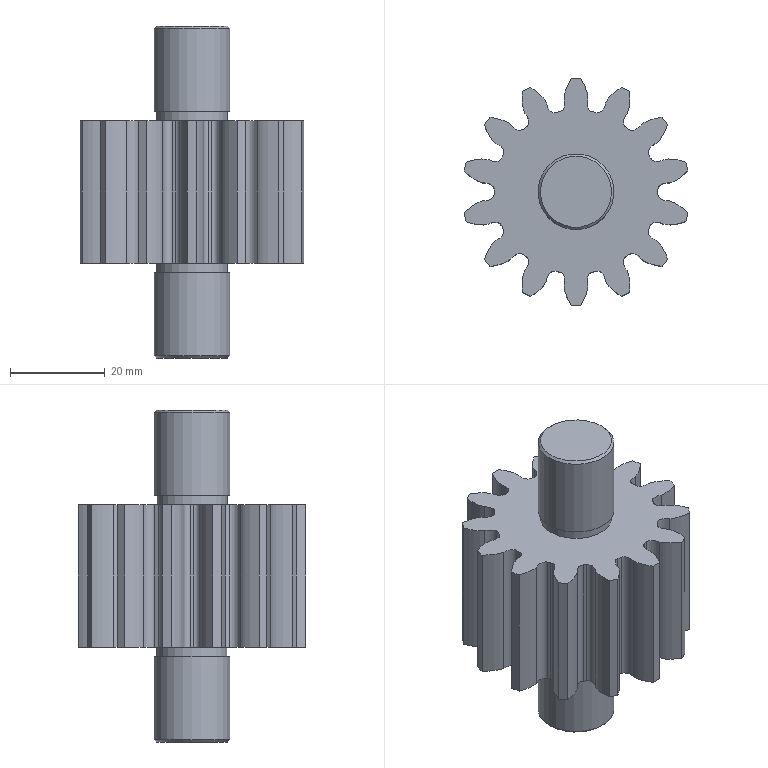Part | NX | features BREP 14, META 14, CYLINDER 3, CHAMFER 2, DATUM_CSYS 2, EXTRACT_FACE 2, EXTRACT_STRING 2, EXTRUDE 2, DATUM_PLANE 1, FSET 1, Instance Feature 1, Mirror Feature 1, SKETCH 1 | 1 solid | 96 faces | box 47.19 x 48 x 70 mm | volume 48349 mm3 | spline 70 | cylinder 18 | plane 6 | cone 2 | commonest cylinder face diameters 34.5 x14 15 x2 16 x2